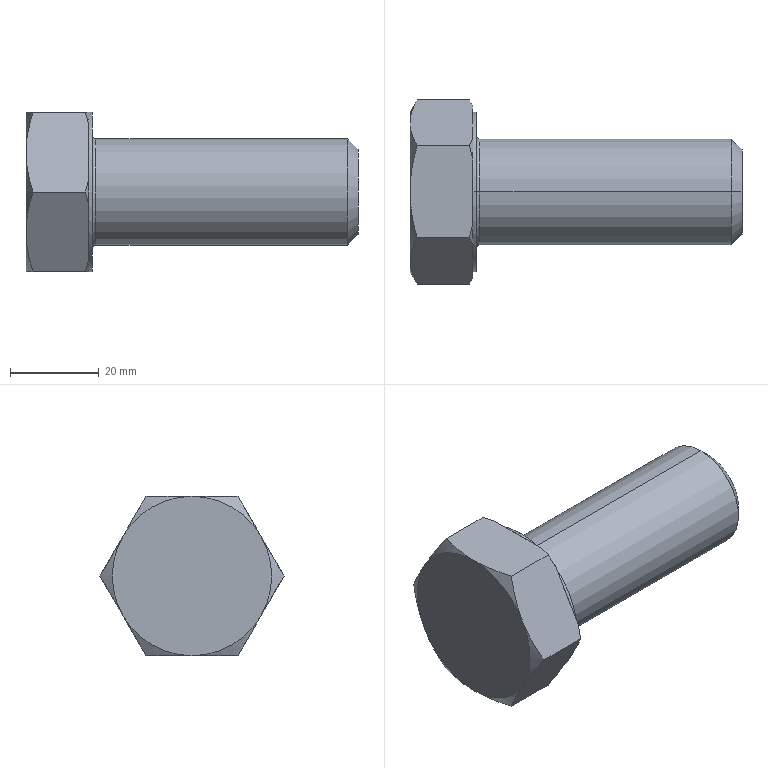Part | STEP file | GB/T 5786-2000 hex head bolt, fine thread, fully threaded, grade A and B, M24×60 (5.6 grade) | 1 solid | 35 faces | box 75 x 41.569 x 36 mm | volume 43647 mm3 | plane 15 | cone 14 | cylinder 4 | torus 2 | commonest cylinder face diameters 24 x2 36 x2